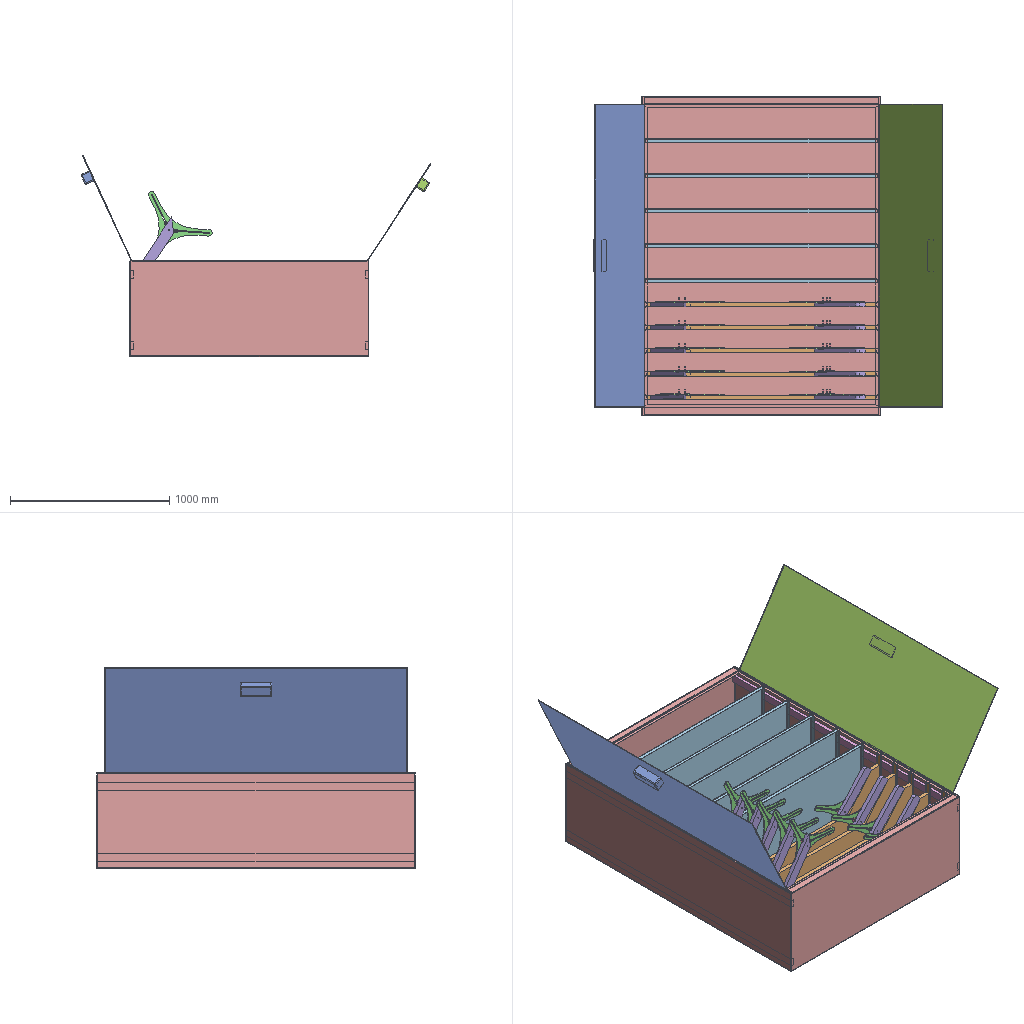Assembly | SolidWorks | 10 different items | 77 placed | box 2195 x 2000 x 1263 mm
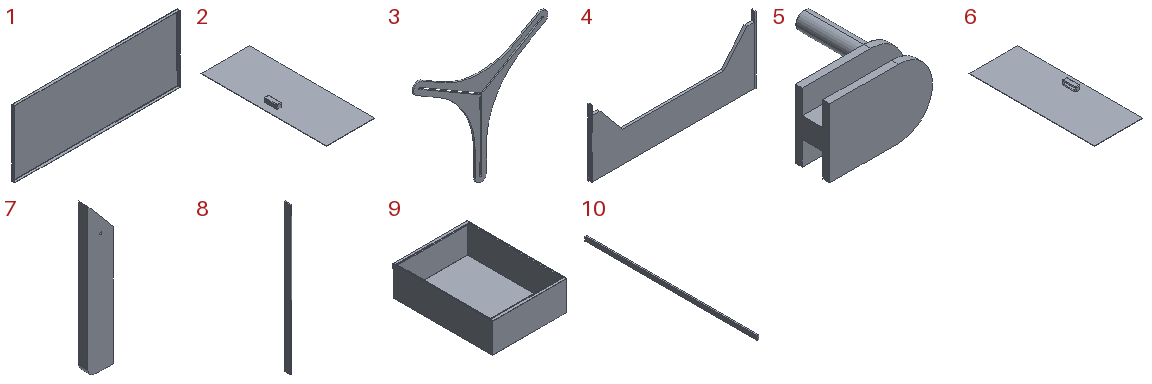Parts list (item | quantity | size | volume | features):
1 | x5 | 1456 x 25 x 590 mm | 1894739 mm3 | features EdgeFlange 1, FlatPattern 1, SMBaseFlange 1, SheetMetal 1
2 | x1 | 735 x 1900 x 64 mm | 3179609 mm3 | features Fillet 3, EdgeFlange 1, FlatPattern 1, ICE 1, SMBaseFlange 1, SheetMetal 1, Shell 1
3 | x10 | 472.147 x 6 x 414.25 mm | 225588 mm3 | features Extrusion 1
4 | x5 | 1456 x 35 x 590 mm | 11968750 mm3 | features Extrusion 1, ICE 1
5 | x30 | 30 x 35 x 20 mm | 3794 mm3 | features ICE 3, Extrusion 1, Fillet 1
6 | x1 | 735 x 1900 x 64 mm | 3179609 mm3 | features Fillet 3, EdgeFlange 1, FlatPattern 1, ICE 1, SMBaseFlange 1, SheetMetal 1, Shell 1
7 | x10 | 67.5 x 25 x 394.016 mm | 594550 mm3 | features Extrusion 1, Fillet 1
8 | x10 | 5 x 25 x 580 mm | 72500 mm3 | features Extrusion 1
9 | x1 | 1500 x 2000 x 600 mm | 14989155 mm3 | features EdgeFlange 6, FlatPattern 1, SMBaseFlange 1, SheetMetal 1, WeldmentFeature 1
10 | x4 | 20 x 1996 x 50 mm | 1996000 mm3 | features Extrusion 1
Mates (type | each side: item.copy, entity, surface, feature):
Coincident | 9.1 face plane Edge-Flange1 | 10.1 face plane Boss-Extrude1 | 2 times
Coincident | 10.1 face plane Boss-Extrude1 | 8.1 face plane Boss-Extrude1
Coincident | 9.1 face plane Base-Flange1 | 8.1 face plane Boss-Extrude1
DistanceDim | 8.1 face plane Boss-Extrude1 | 9.1 face plane Edge-Flange1
Coincident | 9.1 face plane Base-Flange1 | 8.2 face plane Boss-Extrude1
Coincident | 8.1 face plane Boss-Extrude1 | 8.2 face plane Boss-Extrude1
Coincident | assembly face | 8.2 face plane Boss-Extrude1
Coincident | 8.1 face plane Boss-Extrude1 | 4.1 face plane Boss-Extrude1 | 2 times
Coincident | 4.1 edge | 7.1 edge
Coincident | 4.1 face plane Boss-Extrude1 | 7.1 face plane Boss-Extrude1
Coincident | 9.1 face plane Base-Flange1 | 4.1 face plane Boss-Extrude1
Coincident | 7.1 face plane Boss-Extrude1 | 3.1 face plane Boss-Extrude2
Concentric | 7.1 face cylinder Boss-Extrude1 | 3.1 face cylinder Boss-Extrude2
Coincident | 3.1 face plane Boss-Extrude2 | 5.1 face plane Cut-Extrude1 | 2 times
Coincident | 3.1 face plane Boss-Extrude2 | 5.2 face plane Cut-Extrude1 | 2 times
Coincident | 3.1 face plane Boss-Extrude2 | 5.3 face plane Cut-Extrude1 | 2 times
Coincident | 4.1 face plane Boss-Extrude1 | 7.2 face plane Boss-Extrude1
Coincident | 4.1 edge | 7.2 edge
Concentric | 7.2 face cylinder Boss-Extrude1 | 3.2 face cylinder Boss-Extrude2
Coincident | 7.2 face plane Boss-Extrude1 | 3.2 face plane Boss-Extrude2
DistanceDim | 5.1 face cylinder Boss-Extrude2 | 3.1 face cylinder Boss-Extrude2
DistanceDim | 5.3 face cylinder Boss-Extrude2 | 3.1 face cylinder Boss-Extrude2
DistanceDim | 5.2 face cylinder Boss-Extrude2 | 3.1 face cylinder Boss-Extrude2
Coincident | 3.2 face plane Boss-Extrude2 | 5.4 face plane Cut-Extrude1 | 2 times
DistanceDim | 5.4 face cylinder Boss-Extrude2 | 3.2 face cylinder Boss-Extrude2
Coincident | 3.2 face plane Boss-Extrude2 | 5.5 face plane Cut-Extrude1 | 2 times
DistanceDim | 5.5 face cylinder Boss-Extrude2 | 3.2 face cylinder Boss-Extrude2
Coincident | 3.2 face plane Boss-Extrude2 | 5.6 face plane Cut-Extrude1 | 2 times
DistanceDim | 5.6 face cylinder Boss-Extrude2 | 3.2 face cylinder Boss-Extrude2
Coincident | 9.1 face plane Base-Flange1 | 1.1 face plane Edge-Flange1
Coincident | assembly face | 1.1 face plane Edge-Flange1
Parallel | 3.3 face plane Boss-Extrude2 | 4.2 face plane Boss-Extrude1
Coincident | 7.3 edge | 4.2 face plane Cut-Extrude1
DistanceDim | 1.1 face plane Edge-Flange1 | 4.2 face plane Boss-Extrude1
Coincident | 9.1 face plane Edge-Flange7 | 2.1 face plane Edge-Flange1
Coincident | 9.1 edge | 2.1 edge
Coincident | 9.1 face plane Edge-Flange7 | 6.1 face plane Edge-Flange1
Coincident | 9.1 edge | 6.1 edge
Coincident | 10.1 face plane Boss-Extrude1 | 10.2 face plane Boss-Extrude1 | 2 times
Coincident | 8.2 face plane Boss-Extrude1 | 10.2 face plane Boss-Extrude1
Coincident | 10.1 face plane Boss-Extrude1 | 10.3 face plane Boss-Extrude1
Coincident | 10.4 face plane Boss-Extrude1 | 10.3 face plane Boss-Extrude1
Coincident | 10.2 face plane Boss-Extrude1 | 10.3 face plane Boss-Extrude1